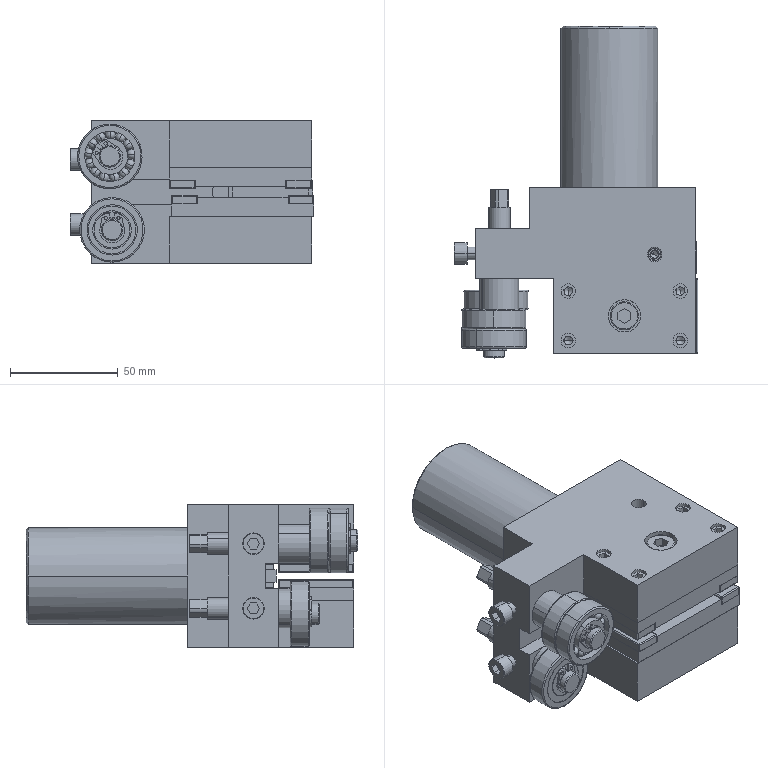Part | SolidWorks | features ReferencePattern 4, MirrorCompFeat 1 | 77 solids | 847 faces | box 113.1 x 154 x 66 mm | volume 527835 mm3 | plane 318 | cylinder 259 | cone 116 | sphere 96 | torus 58 | commonest cylinder face diameters 1 x36 10 x30 6.8 x22 8 x22 16.667 x18 23.333 x18